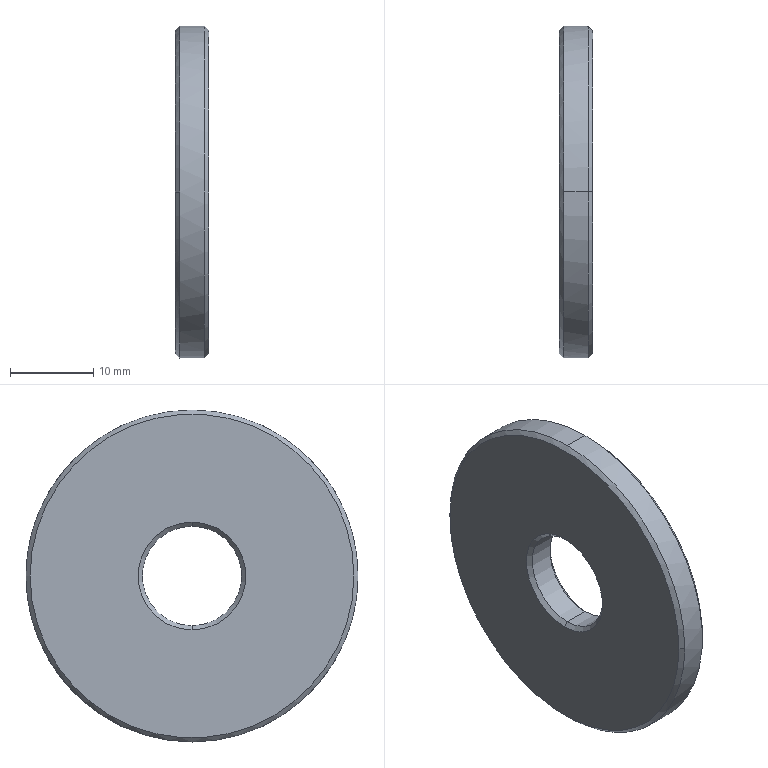Part | SolidWorks | features BaseBody 1 | 1 solid | 14 faces | box 4 x 40 x 40 mm | volume 4533 mm3 | cone 8 | cylinder 4 | plane 2 | commonest cylinder face diameters 12 x2 40 x2
STEP:
#1=CARTESIAN_POINT('',(3.5,0.,6.));
#2=VERTEX_POINT('',#1);
#3=CARTESIAN_POINT('',(3.5,0.,-6.));
#4=VERTEX_POINT('',#3);
#5=CARTESIAN_POINT('',(3.5,0.,0.));
#6=DIRECTION('',(1.,0.,0.));
#7=DIRECTION('',(0.,0.,-1.));
#8=AXIS2_PLACEMENT_3D('',#5,#6,#7);
#9=CIRCLE('',#8,6.);
#10=EDGE_CURVE('',#2,#4,#9,.T.);
#11=ORIENTED_EDGE('',*,*,#10,.F.);
#12=CARTESIAN_POINT('',(4.,0.,6.5));
#13=VERTEX_POINT('',#12);
#14=CARTESIAN_POINT('',(4.,0.,6.5));
#15=DIRECTION('',(0.7071,0.,0.7071));
#16=VECTOR('',#15,1000.);
#17=LINE('',#14,#16);
#18=EDGE_CURVE('',#2,#13,#17,.T.);
#19=ORIENTED_EDGE('',*,*,#18,.T.);
#20=CARTESIAN_POINT('',(4.,0.,-6.5));
#21=VERTEX_POINT('',#20);
#22=CARTESIAN_POINT('',(4.,0.,0.));
#23=DIRECTION('',(-1.,0.,0.));
#24=DIRECTION('',(0.,0.,-1.));
#25=AXIS2_PLACEMENT_3D('',#22,#23,#24);
#26=CIRCLE('',#25,6.5);
#27=EDGE_CURVE('',#21,#13,#26,.T.);
#28=ORIENTED_EDGE('',*,*,#27,.F.);
#29=CARTESIAN_POINT('',(4.,0.,-6.5));
#30=DIRECTION('',(0.7071,0.,-0.7071));
#31=VECTOR('',#30,1000.);
#32=LINE('',#29,#31);
#33=EDGE_CURVE('',#4,#21,#32,.T.);
#34=ORIENTED_EDGE('',*,*,#33,.F.);
#35=EDGE_LOOP('',(#11,#19,#28,#34));
#36=FACE_OUTER_BOUND('',#35,.T.);
#37=CARTESIAN_POINT('',(4.,0.,0.));
#38=DIRECTION('',(1.,0.,0.));
#39=DIRECTION('',(0.,0.,-1.));
#40=AXIS2_PLACEMENT_3D('',#37,#38,#39);
#41=CONICAL_SURFACE('',#40,6.5,0.7854);
#42=ADVANCED_FACE('',(#36),#41,.F.);
#43=CARTESIAN_POINT('',(4.,0.,-19.5));
#44=VERTEX_POINT('',#43);
#45=CARTESIAN_POINT('',(4.,0.,19.5));
#46=VERTEX_POINT('',#45);
#47=CARTESIAN_POINT('',(4.,0.,0.));
#48=DIRECTION('',(1.,0.,0.));
#49=DIRECTION('',(0.,0.,1.));
#50=AXIS2_PLACEMENT_3D('',#47,#48,#49);
#51=CIRCLE('',#50,19.5);
#52=EDGE_CURVE('',#44,#46,#51,.T.);
#53=ORIENTED_EDGE('',*,*,#52,.F.);
#54=CARTESIAN_POINT('',(3.5,0.,-20.));
#55=VERTEX_POINT('',#54);
#56=CARTESIAN_POINT('',(3.5,0.,-20.));
#57=DIRECTION('',(-0.7071,0.,-0.7071));
#58=VECTOR('',#57,1000.);
#59=LINE('',#56,#58);
#60=EDGE_CURVE('',#44,#55,#59,.T.);
#61=ORIENTED_EDGE('',*,*,#60,.T.);
#62=CARTESIAN_POINT('',(3.5,0.,20.));
#63=VERTEX_POINT('',#62);
#64=CARTESIAN_POINT('',(3.5,0.,0.));
#65=DIRECTION('',(1.,0.,0.));
#66=DIRECTION('',(0.,0.,-1.));
#67=AXIS2_PLACEMENT_3D('',#64,#65,#66);
#68=CIRCLE('',#67,20.);
#69=EDGE_CURVE('',#55,#63,#68,.T.);
#70=ORIENTED_EDGE('',*,*,#69,.T.);
#71=CARTESIAN_POINT('',(3.5,0.,20.));
#72=DIRECTION('',(-0.7071,0.,0.7071));
#73=VECTOR('',#72,1000.);
#74=LINE('',#71,#73);
#75=EDGE_CURVE('',#46,#63,#74,.T.);
#76=ORIENTED_EDGE('',*,*,#75,.F.);
#77=EDGE_LOOP('',(#53,#61,#70,#76));
#78=FACE_OUTER_BOUND('',#77,.T.);
#79=CARTESIAN_POINT('',(3.5,0.,0.));
#80=DIRECTION('',(-1.,0.,0.));
#81=DIRECTION('',(0.,0.,1.));
#82=AXIS2_PLACEMENT_3D('',#79,#80,#81);
#83=CONICAL_SURFACE('',#82,20.,0.7854);
#84=ADVANCED_FACE('',(#78),#83,.T.);
#85=CARTESIAN_POINT('',(0.5,0.,6.));
#86=VERTEX_POINT('',#85);
#87=CARTESIAN_POINT('',(0.5,0.,-6.));
#88=VERTEX_POINT('',#87);
#89=CARTESIAN_POINT('',(0.5,0.,0.));
#90=DIRECTION('',(1.,0.,0.));
#91=DIRECTION('',(0.,0.,-1.));
#92=AXIS2_PLACEMENT_3D('',#89,#90,#91);
#93=CIRCLE('',#92,6.);
#94=EDGE_CURVE('',#86,#88,#93,.T.);
#95=ORIENTED_EDGE('',*,*,#94,.F.);
#96=CARTESIAN_POINT('',(0.,0.,6.));
#97=DIRECTION('',(1.,0.,0.));
#98=VECTOR('',#97,1000.);
#99=LINE('',#96,#98);
#100=EDGE_CURVE('',#86,#2,#99,.T.);
#101=ORIENTED_EDGE('',*,*,#100,.T.);
#102=ORIENTED_EDGE('',*,*,#10,.T.);
#103=CARTESIAN_POINT('',(0.,0.,-6.));
#104=DIRECTION('',(1.,0.,0.));
#105=VECTOR('',#104,1000.);
#106=LINE('',#103,#105);
#107=EDGE_CURVE('',#88,#4,#106,.T.);
#108=ORIENTED_EDGE('',*,*,#107,.F.);
#109=EDGE_LOOP('',(#95,#101,#102,#108));
#110=FACE_OUTER_BOUND('',#109,.T.);
#111=CARTESIAN_POINT('',(0.,0.,0.));
#112=DIRECTION('',(1.,0.,0.));
#113=DIRECTION('',(0.,0.,-1.));
#114=AXIS2_PLACEMENT_3D('',#111,#112,#113);
#115=CYLINDRICAL_SURFACE('',#114,6.);
#116=ADVANCED_FACE('',(#110),#115,.F.);
#117=CARTESIAN_POINT('',(0.5,20.,0.));
#118=VERTEX_POINT('',#117);
#119=CARTESIAN_POINT('',(0.5,0.,20.));
#120=VERTEX_POINT('',#119);
#121=CARTESIAN_POINT('',(0.5,0.,0.));
#122=DIRECTION('',(1.,0.,0.));
#123=DIRECTION('',(0.,0.,-1.));
#124=AXIS2_PLACEMENT_3D('',#121,#122,#123);
#125=CIRCLE('',#124,20.);
#126=EDGE_CURVE('',#118,#120,#125,.T.);
#127=ORIENTED_EDGE('',*,*,#126,.T.);
#128=CARTESIAN_POINT('',(0.,0.,20.));
#129=DIRECTION('',(1.,0.,0.));
#130=VECTOR('',#129,1000.);
#131=LINE('',#128,#130);
#132=EDGE_CURVE('',#120,#63,#131,.T.);
#133=ORIENTED_EDGE('',*,*,#132,.T.);
#134=ORIENTED_EDGE('',*,*,#69,.F.);
#135=CARTESIAN_POINT('',(0.5,0.,-20.));
#136=VERTEX_POINT('',#135);
#137=CARTESIAN_POINT('',(0.,0.,-20.));
#138=DIRECTION('',(1.,0.,0.));
#139=VECTOR('',#138,1000.);
#140=LINE('',#137,#139);
#141=EDGE_CURVE('',#136,#55,#140,.T.);
#142=ORIENTED_EDGE('',*,*,#141,.F.);
#143=CARTESIAN_POINT('',(0.5,0.,0.));
#144=DIRECTION('',(1.,0.,0.));
#145=DIRECTION('',(0.,0.,-1.));
#146=AXIS2_PLACEMENT_3D('',#143,#144,#145);
#147=CIRCLE('',#146,20.);
#148=EDGE_CURVE('',#136,#118,#147,.T.);
#149=ORIENTED_EDGE('',*,*,#148,.T.);
#150=EDGE_LOOP('',(#127,#133,#134,#142,#149));
#151=FACE_OUTER_BOUND('',#150,.T.);
#152=CARTESIAN_POINT('',(0.,0.,0.));
#153=DIRECTION('',(1.,0.,0.));
#154=DIRECTION('',(0.,0.,-1.));
#155=AXIS2_PLACEMENT_3D('',#152,#153,#154);
#156=CYLINDRICAL_SURFACE('',#155,20.);
#157=ADVANCED_FACE('',(#151),#156,.T.);
#158=ORIENTED_EDGE('',*,*,#94,.T.);
#159=CARTESIAN_POINT('',(0.,0.,-6.5));
#160=VERTEX_POINT('',#159);
#161=CARTESIAN_POINT('',(0.,0.,-6.5));
#162=DIRECTION('',(-0.7071,0.,-0.7071));
#163=VECTOR('',#162,1000.);
#164=LINE('',#161,#163);
#165=EDGE_CURVE('',#88,#160,#164,.T.);
#166=ORIENTED_EDGE('',*,*,#165,.T.);
#167=CARTESIAN_POINT('',(0.,0.,6.5));
#168=VERTEX_POINT('',#167);
#169=CARTESIAN_POINT('',(0.,0.,0.));
#170=DIRECTION('',(1.,0.,0.));
#171=DIRECTION('',(0.,0.,1.));
#172=AXIS2_PLACEMENT_3D('',#169,#170,#171);
#173=CIRCLE('',#172,6.5);
#174=EDGE_CURVE('',#168,#160,#173,.T.);
#175=ORIENTED_EDGE('',*,*,#174,.F.);
#176=CARTESIAN_POINT('',(0.,0.,6.5));
#177=DIRECTION('',(-0.7071,0.,0.7071));
#178=VECTOR('',#177,1000.);
#179=LINE('',#176,#178);
#180=EDGE_CURVE('',#86,#168,#179,.T.);
#181=ORIENTED_EDGE('',*,*,#180,.F.);
#182=EDGE_LOOP('',(#158,#166,#175,#181));
#183=FACE_OUTER_BOUND('',#182,.T.);
#184=CARTESIAN_POINT('',(0.,0.,0.));
#185=DIRECTION('',(-1.,0.,0.));
#186=DIRECTION('',(0.,0.,1.));
#187=AXIS2_PLACEMENT_3D('',#184,#185,#186);
#188=CONICAL_SURFACE('',#187,6.5,0.7854);
#189=ADVANCED_FACE('',(#183),#188,.F.);
#190=CARTESIAN_POINT('',(0.,19.5,0.));
#191=VERTEX_POINT('',#190);
#192=CARTESIAN_POINT('',(0.,-19.5,0.));
#193=VERTEX_POINT('',#192);
#194=CARTESIAN_POINT('',(0.,0.,0.));
#195=DIRECTION('',(1.,0.,0.));
#196=DIRECTION('',(0.,1.,0.));
#197=AXIS2_PLACEMENT_3D('',#194,#195,#196);
#198=CIRCLE('',#197,19.5);
#199=EDGE_CURVE('',#191,#193,#198,.T.);
#200=ORIENTED_EDGE('',*,*,#199,.T.);
#201=CARTESIAN_POINT('',(0.5,-20.,0.));
#202=VERTEX_POINT('',#201);
#203=CARTESIAN_POINT('',(0.5,-20.,0.));
#204=DIRECTION('',(0.7071,-0.7071,0.));
#205=VECTOR('',#204,1000.);
#206=LINE('',#203,#205);
#207=EDGE_CURVE('',#193,#202,#206,.T.);
#208=ORIENTED_EDGE('',*,*,#207,.T.);
#209=CARTESIAN_POINT('',(0.5,0.,0.));
#210=DIRECTION('',(1.,0.,0.));
#211=DIRECTION('',(0.,0.,-1.));
#212=AXIS2_PLACEMENT_3D('',#209,#210,#211);
#213=CIRCLE('',#212,20.);
#214=EDGE_CURVE('',#120,#202,#213,.T.);
#215=ORIENTED_EDGE('',*,*,#214,.F.);
#216=ORIENTED_EDGE('',*,*,#126,.F.);
#217=CARTESIAN_POINT('',(0.5,20.,0.));
#218=DIRECTION('',(0.7071,0.7071,0.));
#219=VECTOR('',#218,1000.);
#220=LINE('',#217,#219);
#221=EDGE_CURVE('',#191,#118,#220,.T.);
#222=ORIENTED_EDGE('',*,*,#221,.F.);
#223=EDGE_LOOP('',(#200,#208,#215,#216,#222));
#224=FACE_OUTER_BOUND('',#223,.T.);
#225=CARTESIAN_POINT('',(0.5,0.,0.));
#226=DIRECTION('',(1.,0.,0.));
#227=DIRECTION('',(0.,1.,0.));
#228=AXIS2_PLACEMENT_3D('',#225,#226,#227);
#229=CONICAL_SURFACE('',#228,20.,0.7854);
#230=ADVANCED_FACE('',(#224),#229,.T.);
#231=ORIENTED_EDGE('',*,*,#27,.T.);
#232=CARTESIAN_POINT('',(4.,0.,0.));
#233=DIRECTION('',(-1.,0.,0.));
#234=DIRECTION('',(0.,0.,-1.));
#235=AXIS2_PLACEMENT_3D('',#232,#233,#234);
#236=CIRCLE('',#235,6.5);
#237=EDGE_CURVE('',#13,#21,#236,.T.);
#238=ORIENTED_EDGE('',*,*,#237,.T.);
#239=EDGE_LOOP('',(#231,#238));
#240=FACE_BOUND('',#239,.T.);
#241=CARTESIAN_POINT('',(4.,0.,0.));
#242=DIRECTION('',(1.,0.,0.));
#243=DIRECTION('',(0.,0.,1.));
#244=AXIS2_PLACEMENT_3D('',#241,#242,#243);
#245=CIRCLE('',#244,19.5);
#246=EDGE_CURVE('',#46,#44,#245,.T.);
#247=ORIENTED_EDGE('',*,*,#246,.T.);
#248=ORIENTED_EDGE('',*,*,#52,.T.);
#249=EDGE_LOOP('',(#247,#248));
#250=FACE_OUTER_BOUND('',#249,.T.);
#251=CARTESIAN_POINT('',(4.,0.,0.));
#252=DIRECTION('',(1.,0.,0.));
#253=DIRECTION('',(0.,0.,-1.));
#254=AXIS2_PLACEMENT_3D('',#251,#252,#253);
#255=PLANE('',#254);
#256=ADVANCED_FACE('',(#240,#250),#255,.T.);
#257=ORIENTED_EDGE('',*,*,#18,.F.);
#258=CARTESIAN_POINT('',(3.5,0.,0.));
#259=DIRECTION('',(1.,0.,0.));
#260=DIRECTION('',(0.,0.,-1.));
#261=AXIS2_PLACEMENT_3D('',#258,#259,#260);
#262=CIRCLE('',#261,6.);
#263=EDGE_CURVE('',#4,#2,#262,.T.);
#264=ORIENTED_EDGE('',*,*,#263,.F.);
#265=ORIENTED_EDGE('',*,*,#33,.T.);
#266=ORIENTED_EDGE('',*,*,#237,.F.);
#267=EDGE_LOOP('',(#257,#264,#265,#266));
#268=FACE_OUTER_BOUND('',#267,.T.);
#269=CARTESIAN_POINT('',(4.,0.,0.));
#270=DIRECTION('',(1.,0.,0.));
#271=DIRECTION('',(0.,0.,-1.));
#272=AXIS2_PLACEMENT_3D('',#269,#270,#271);
#273=CONICAL_SURFACE('',#272,6.5,0.7854);
#274=ADVANCED_FACE('',(#268),#273,.F.);
#275=ORIENTED_EDGE('',*,*,#60,.F.);
#276=ORIENTED_EDGE('',*,*,#246,.F.);
#277=ORIENTED_EDGE('',*,*,#75,.T.);
#278=CARTESIAN_POINT('',(3.5,0.,0.));
#279=DIRECTION('',(1.,0.,0.));
#280=DIRECTION('',(0.,0.,-1.));
#281=AXIS2_PLACEMENT_3D('',#278,#279,#280);
#282=CIRCLE('',#281,20.);
#283=EDGE_CURVE('',#63,#55,#282,.T.);
#284=ORIENTED_EDGE('',*,*,#283,.T.);
#285=EDGE_LOOP('',(#275,#276,#277,#284));
#286=FACE_OUTER_BOUND('',#285,.T.);
#287=CARTESIAN_POINT('',(3.5,0.,0.));
#288=DIRECTION('',(-1.,0.,0.));
#289=DIRECTION('',(0.,0.,1.));
#290=AXIS2_PLACEMENT_3D('',#287,#288,#289);
#291=CONICAL_SURFACE('',#290,20.,0.7854);
#292=ADVANCED_FACE('',(#286),#291,.T.);
#293=ORIENTED_EDGE('',*,*,#100,.F.);
#294=CARTESIAN_POINT('',(0.5,0.,0.));
#295=DIRECTION('',(1.,0.,0.));
#296=DIRECTION('',(0.,0.,-1.));
#297=AXIS2_PLACEMENT_3D('',#294,#295,#296);
#298=CIRCLE('',#297,6.);
#299=EDGE_CURVE('',#88,#86,#298,.T.);
#300=ORIENTED_EDGE('',*,*,#299,.F.);
#301=ORIENTED_EDGE('',*,*,#107,.T.);
#302=ORIENTED_EDGE('',*,*,#263,.T.);
#303=EDGE_LOOP('',(#293,#300,#301,#302));
#304=FACE_OUTER_BOUND('',#303,.T.);
#305=CARTESIAN_POINT('',(0.,0.,0.));
#306=DIRECTION('',(1.,0.,0.));
#307=DIRECTION('',(0.,0.,-1.));
#308=AXIS2_PLACEMENT_3D('',#305,#306,#307);
#309=CYLINDRICAL_SURFACE('',#308,6.);
#310=ADVANCED_FACE('',(#304),#309,.F.);
#311=ORIENTED_EDGE('',*,*,#132,.F.);
#312=ORIENTED_EDGE('',*,*,#214,.T.);
#313=CARTESIAN_POINT('',(0.5,0.,0.));
#314=DIRECTION('',(1.,0.,0.));
#315=DIRECTION('',(0.,0.,-1.));
#316=AXIS2_PLACEMENT_3D('',#313,#314,#315);
#317=CIRCLE('',#316,20.);
#318=EDGE_CURVE('',#202,#136,#317,.T.);
#319=ORIENTED_EDGE('',*,*,#318,.T.);
#320=ORIENTED_EDGE('',*,*,#141,.T.);
#321=ORIENTED_EDGE('',*,*,#283,.F.);
#322=EDGE_LOOP('',(#311,#312,#319,#320,#321));
#323=FACE_OUTER_BOUND('',#322,.T.);
#324=CARTESIAN_POINT('',(0.,0.,0.));
#325=DIRECTION('',(1.,0.,0.));
#326=DIRECTION('',(0.,0.,-1.));
#327=AXIS2_PLACEMENT_3D('',#324,#325,#326);
#328=CYLINDRICAL_SURFACE('',#327,20.);
#329=ADVANCED_FACE('',(#323),#328,.T.);
#330=ORIENTED_EDGE('',*,*,#165,.F.);
#331=ORIENTED_EDGE('',*,*,#299,.T.);
#332=ORIENTED_EDGE('',*,*,#180,.T.);
#333=CARTESIAN_POINT('',(0.,0.,0.));
#334=DIRECTION('',(1.,0.,0.));
#335=DIRECTION('',(0.,0.,1.));
#336=AXIS2_PLACEMENT_3D('',#333,#334,#335);
#337=CIRCLE('',#336,6.5);
#338=EDGE_CURVE('',#160,#168,#337,.T.);
#339=ORIENTED_EDGE('',*,*,#338,.F.);
#340=EDGE_LOOP('',(#330,#331,#332,#339));
#341=FACE_OUTER_BOUND('',#340,.T.);
#342=CARTESIAN_POINT('',(0.,0.,0.));
#343=DIRECTION('',(-1.,0.,0.));
#344=DIRECTION('',(0.,0.,1.));
#345=AXIS2_PLACEMENT_3D('',#342,#343,#344);
#346=CONICAL_SURFACE('',#345,6.5,0.7854);
#347=ADVANCED_FACE('',(#341),#346,.F.);
#348=ORIENTED_EDGE('',*,*,#207,.F.);
#349=CARTESIAN_POINT('',(0.,0.,0.));
#350=DIRECTION('',(1.,0.,0.));
#351=DIRECTION('',(0.,1.,0.));
#352=AXIS2_PLACEMENT_3D('',#349,#350,#351);
#353=CIRCLE('',#352,19.5);
#354=EDGE_CURVE('',#193,#191,#353,.T.);
#355=ORIENTED_EDGE('',*,*,#354,.T.);
#356=ORIENTED_EDGE('',*,*,#221,.T.);
#357=ORIENTED_EDGE('',*,*,#148,.F.);
#358=ORIENTED_EDGE('',*,*,#318,.F.);
#359=EDGE_LOOP('',(#348,#355,#356,#357,#358));
#360=FACE_OUTER_BOUND('',#359,.T.);
#361=CARTESIAN_POINT('',(0.5,0.,0.));
#362=DIRECTION('',(1.,0.,0.));
#363=DIRECTION('',(0.,1.,0.));
#364=AXIS2_PLACEMENT_3D('',#361,#362,#363);
#365=CONICAL_SURFACE('',#364,20.,0.7854);
#366=ADVANCED_FACE('',(#360),#365,.T.);
#367=ORIENTED_EDGE('',*,*,#174,.T.);
#368=ORIENTED_EDGE('',*,*,#338,.T.);
#369=EDGE_LOOP('',(#367,#368));
#370=FACE_BOUND('',#369,.T.);
#371=ORIENTED_EDGE('',*,*,#199,.F.);
#372=ORIENTED_EDGE('',*,*,#354,.F.);
#373=EDGE_LOOP('',(#371,#372));
#374=FACE_OUTER_BOUND('',#373,.T.);
#375=CARTESIAN_POINT('',(0.,0.,0.));
#376=DIRECTION('',(1.,0.,0.));
#377=DIRECTION('',(0.,0.,-1.));
#378=AXIS2_PLACEMENT_3D('',#375,#376,#377);
#379=PLANE('',#378);
#380=ADVANCED_FACE('',(#370,#374),#379,.F.);
#381=CLOSED_SHELL('',(#42,#84,#116,#157,#189,#230,#256,#274,#292,#310,#329,#347,#366,#380));
#382=MANIFOLD_SOLID_BREP('',#381);
#383=CARTESIAN_POINT('',(0.,0.,0.));
#384=DIRECTION('',(0.,0.,1.));
#385=DIRECTION('',(1.,0.,0.));
#386=AXIS2_PLACEMENT_3D('',#383,#384,#385);
#387=(LENGTH_UNIT()NAMED_UNIT(*)SI_UNIT(.MILLI.,.METRE.));
#388=UNCERTAINTY_MEASURE_WITH_UNIT(LENGTH_MEASURE(0.00001),#387,'','');
#389=(NAMED_UNIT(*)PLANE_ANGLE_UNIT()SI_UNIT($,.RADIAN.));
#390=(NAMED_UNIT(*)SI_UNIT($,.STERADIAN.)SOLID_ANGLE_UNIT());
#391=(GEOMETRIC_REPRESENTATION_CONTEXT(3)GLOBAL_UNCERTAINTY_ASSIGNED_CONTEXT((#388))GLOBAL_UNIT_ASSIGNED_CONTEXT((#387,#389,#390))REPRESENTATION_CONTEXT('',''));
#392=ADVANCED_BREP_SHAPE_REPRESENTATION('',(#382,#386),#391);